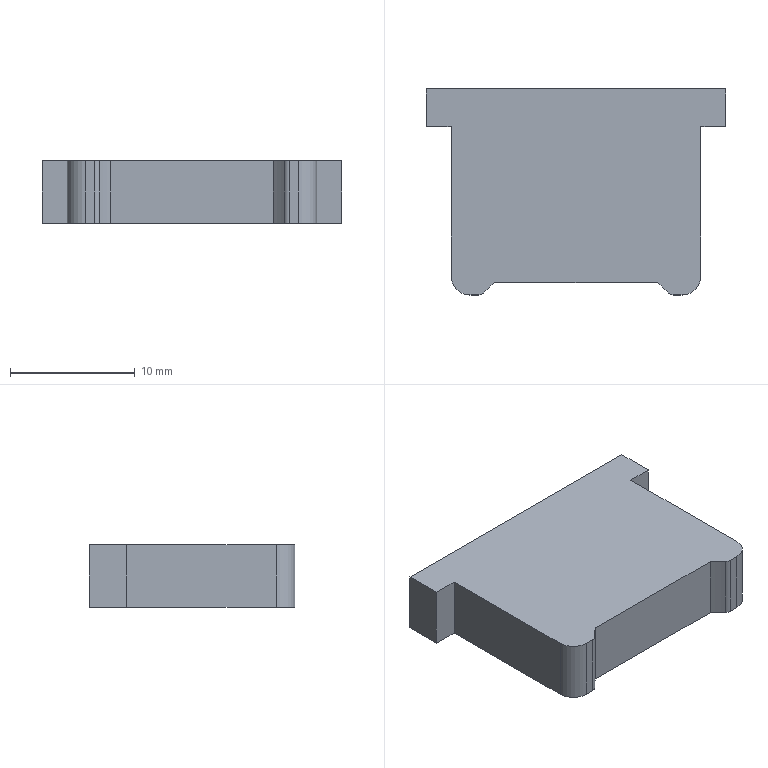Part | STEP file | iron shell positioning insert | 1 solid | 21 faces | box 24 x 16.5 x 5 mm | volume 1571 mm3 | plane 13 | cylinder 8 | commonest cylinder face diameters 1 x2 3 x2 4.5 x2 20.6 x2